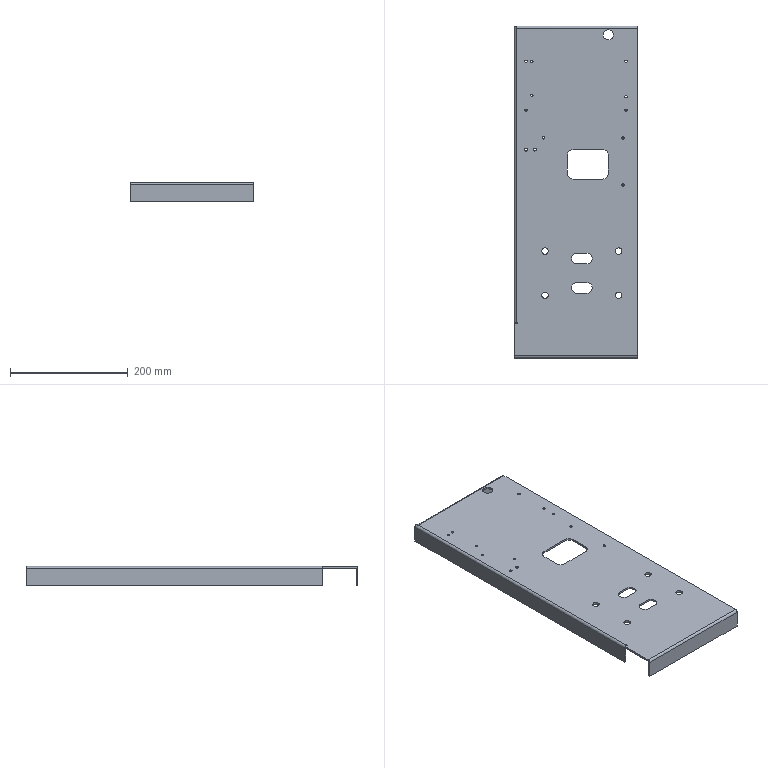Part | STEP file | PN_0005 default | 1 solid | 68 faces | box 210 x 564 x 33 mm | volume 419212 mm3 | plane 37 | cylinder 31 | commonest cylinder face diameters 4 x10 11 x4 18 x4 20 x4 2 x3 8 x3